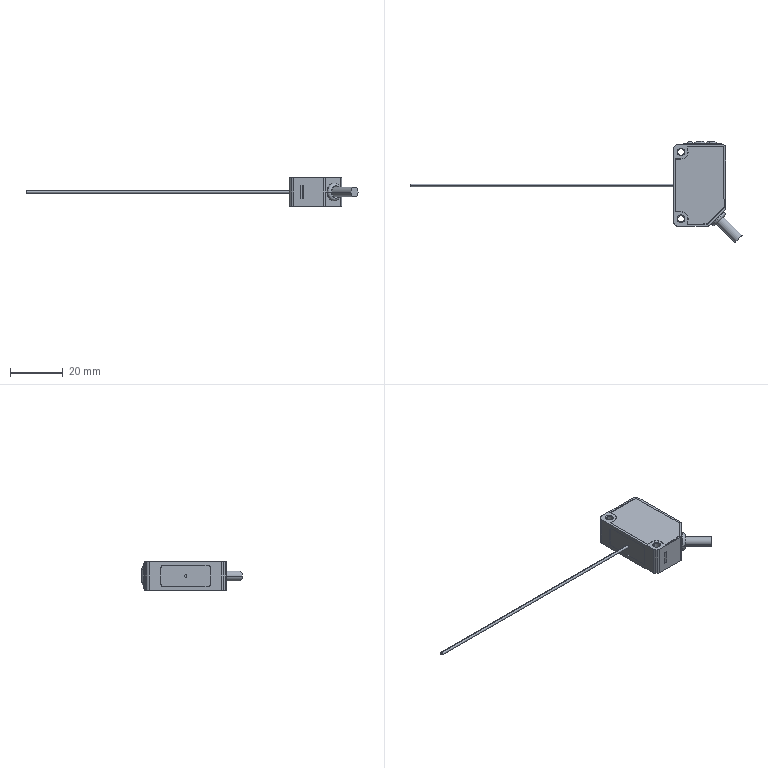Part | SolidWorks | features BaseBody 1, ICE 1 | 1 solid | 212 faces | box 126.19 x 38.39 x 11 mm | volume 6688 mm3 | plane 115 | cylinder 79 | torus 8 | cone 8 | sphere 2 | commonest cylinder face diameters 2 x9 4.02 x8 2.4 x7 2.3 x6 0.8 x4 1.6 x4